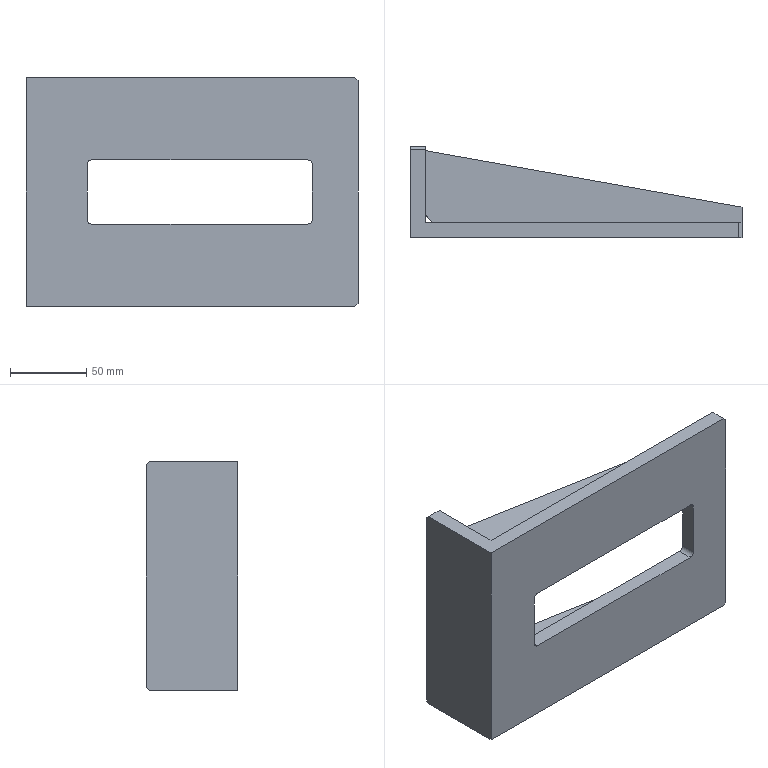Part | SolidWorks | features ICE 2, Chamfer 1, Extrusion 1, Fillet 1, MirrorPattern 1 | 1 solid | 28 faces | box 217.5 x 60 x 150 mm | volume 433717 mm3 | plane 24 | cylinder 4 | commonest cylinder face diameters 6 x4
STEP:
#1=CARTESIAN_POINT('',(0.,58.,75.));
#2=VERTEX_POINT('',#1);
#3=CARTESIAN_POINT('',(0.,0.,75.));
#4=VERTEX_POINT('',#3);
#5=CARTESIAN_POINT('',(0.,60.,75.));
#6=DIRECTION('',(0.,-1.,0.));
#7=VECTOR('',#6,1000.);
#8=LINE('',#5,#7);
#9=EDGE_CURVE('',#2,#4,#8,.T.);
#10=ORIENTED_EDGE('',*,*,#9,.F.);
#11=CARTESIAN_POINT('',(0.,60.,73.));
#12=VERTEX_POINT('',#11);
#13=CARTESIAN_POINT('',(0.,58.,75.));
#14=DIRECTION('',(0.,0.7071,-0.7071));
#15=VECTOR('',#14,1000.);
#16=LINE('',#13,#15);
#17=EDGE_CURVE('',#2,#12,#16,.T.);
#18=ORIENTED_EDGE('',*,*,#17,.T.);
#19=CARTESIAN_POINT('',(0.,60.,-73.));
#20=VERTEX_POINT('',#19);
#21=CARTESIAN_POINT('',(0.,60.,75.));
#22=DIRECTION('',(0.,0.,-1.));
#23=VECTOR('',#22,1000.);
#24=LINE('',#21,#23);
#25=EDGE_CURVE('',#12,#20,#24,.T.);
#26=ORIENTED_EDGE('',*,*,#25,.T.);
#27=CARTESIAN_POINT('',(0.,58.,-75.));
#28=VERTEX_POINT('',#27);
#29=CARTESIAN_POINT('',(0.,60.,-73.));
#30=DIRECTION('',(0.,-0.7071,-0.7071));
#31=VECTOR('',#30,1000.);
#32=LINE('',#29,#31);
#33=EDGE_CURVE('',#20,#28,#32,.T.);
#34=ORIENTED_EDGE('',*,*,#33,.T.);
#35=CARTESIAN_POINT('',(0.,0.,-75.));
#36=VERTEX_POINT('',#35);
#37=CARTESIAN_POINT('',(0.,60.,-75.));
#38=DIRECTION('',(0.,-1.,0.));
#39=VECTOR('',#38,1000.);
#40=LINE('',#37,#39);
#41=EDGE_CURVE('',#28,#36,#40,.T.);
#42=ORIENTED_EDGE('',*,*,#41,.T.);
#43=CARTESIAN_POINT('',(0.,0.,75.));
#44=DIRECTION('',(0.,0.,-1.));
#45=VECTOR('',#44,1000.);
#46=LINE('',#43,#45);
#47=EDGE_CURVE('',#4,#36,#46,.T.);
#48=ORIENTED_EDGE('',*,*,#47,.F.);
#49=EDGE_LOOP('',(#10,#18,#26,#34,#42,#48));
#50=FACE_OUTER_BOUND('',#49,.T.);
#51=CARTESIAN_POINT('',(0.,60.,75.));
#52=DIRECTION('',(1.,0.,0.));
#53=DIRECTION('',(0.,1.,0.));
#54=AXIS2_PLACEMENT_3D('',#51,#52,#53);
#55=PLANE('',#54);
#56=ADVANCED_FACE('',(#50),#55,.F.);
#57=CARTESIAN_POINT('',(184.5,0.,21.));
#58=VERTEX_POINT('',#57);
#59=CARTESIAN_POINT('',(43.,0.,21.));
#60=VERTEX_POINT('',#59);
#61=CARTESIAN_POINT('',(40.,0.,21.));
#62=DIRECTION('',(-1.,0.,0.));
#63=VECTOR('',#62,1000.);
#64=LINE('',#61,#63);
#65=EDGE_CURVE('',#58,#60,#64,.T.);
#66=ORIENTED_EDGE('',*,*,#65,.F.);
#67=CARTESIAN_POINT('',(187.5,0.,18.));
#68=VERTEX_POINT('',#67);
#69=CARTESIAN_POINT('',(184.5,0.,18.));
#70=DIRECTION('',(0.,1.,0.));
#71=DIRECTION('',(0.,0.,1.));
#72=AXIS2_PLACEMENT_3D('',#69,#70,#71);
#73=CIRCLE('',#72,3.);
#74=EDGE_CURVE('',#58,#68,#73,.T.);
#75=ORIENTED_EDGE('',*,*,#74,.T.);
#76=CARTESIAN_POINT('',(187.5,0.,-18.));
#77=VERTEX_POINT('',#76);
#78=CARTESIAN_POINT('',(187.5,0.,21.));
#79=DIRECTION('',(0.,0.,1.));
#80=VECTOR('',#79,1000.);
#81=LINE('',#78,#80);
#82=EDGE_CURVE('',#77,#68,#81,.T.);
#83=ORIENTED_EDGE('',*,*,#82,.F.);
#84=CARTESIAN_POINT('',(184.5,0.,-21.));
#85=VERTEX_POINT('',#84);
#86=CARTESIAN_POINT('',(184.5,0.,-18.));
#87=DIRECTION('',(0.,1.,0.));
#88=DIRECTION('',(0.,0.,1.));
#89=AXIS2_PLACEMENT_3D('',#86,#87,#88);
#90=CIRCLE('',#89,3.);
#91=EDGE_CURVE('',#77,#85,#90,.T.);
#92=ORIENTED_EDGE('',*,*,#91,.T.);
#93=CARTESIAN_POINT('',(43.,0.,-21.));
#94=VERTEX_POINT('',#93);
#95=CARTESIAN_POINT('',(40.,0.,-21.));
#96=DIRECTION('',(1.,0.,0.));
#97=VECTOR('',#96,1000.);
#98=LINE('',#95,#97);
#99=EDGE_CURVE('',#94,#85,#98,.T.);
#100=ORIENTED_EDGE('',*,*,#99,.F.);
#101=CARTESIAN_POINT('',(40.,0.,-18.));
#102=VERTEX_POINT('',#101);
#103=CARTESIAN_POINT('',(43.,0.,-18.));
#104=DIRECTION('',(0.,1.,0.));
#105=DIRECTION('',(0.,0.,1.));
#106=AXIS2_PLACEMENT_3D('',#103,#104,#105);
#107=CIRCLE('',#106,3.);
#108=EDGE_CURVE('',#94,#102,#107,.T.);
#109=ORIENTED_EDGE('',*,*,#108,.T.);
#110=CARTESIAN_POINT('',(40.,0.,18.));
#111=VERTEX_POINT('',#110);
#112=CARTESIAN_POINT('',(40.,0.,21.));
#113=DIRECTION('',(0.,0.,-1.));
#114=VECTOR('',#113,1000.);
#115=LINE('',#112,#114);
#116=EDGE_CURVE('',#111,#102,#115,.T.);
#117=ORIENTED_EDGE('',*,*,#116,.F.);
#118=CARTESIAN_POINT('',(43.,0.,18.));
#119=DIRECTION('',(0.,1.,0.));
#120=DIRECTION('',(0.,0.,1.));
#121=AXIS2_PLACEMENT_3D('',#118,#119,#120);
#122=CIRCLE('',#121,3.);
#123=EDGE_CURVE('',#111,#60,#122,.T.);
#124=ORIENTED_EDGE('',*,*,#123,.T.);
#125=EDGE_LOOP('',(#66,#75,#83,#92,#100,#109,#117,#124));
#126=FACE_BOUND('',#125,.T.);
#127=CARTESIAN_POINT('',(215.5,0.,-75.));
#128=VERTEX_POINT('',#127);
#129=CARTESIAN_POINT('',(0.,0.,-75.));
#130=DIRECTION('',(1.,0.,0.));
#131=VECTOR('',#130,1000.);
#132=LINE('',#129,#131);
#133=EDGE_CURVE('',#36,#128,#132,.T.);
#134=ORIENTED_EDGE('',*,*,#133,.T.);
#135=CARTESIAN_POINT('',(217.5,0.,-73.));
#136=VERTEX_POINT('',#135);
#137=CARTESIAN_POINT('',(217.5,0.,-73.));
#138=DIRECTION('',(0.7071,0.,0.7071));
#139=VECTOR('',#138,1000.);
#140=LINE('',#137,#139);
#141=EDGE_CURVE('',#128,#136,#140,.T.);
#142=ORIENTED_EDGE('',*,*,#141,.T.);
#143=CARTESIAN_POINT('',(217.5,0.,73.));
#144=VERTEX_POINT('',#143);
#145=CARTESIAN_POINT('',(217.5,0.,75.));
#146=DIRECTION('',(0.,0.,-1.));
#147=VECTOR('',#146,1000.);
#148=LINE('',#145,#147);
#149=EDGE_CURVE('',#144,#136,#148,.T.);
#150=ORIENTED_EDGE('',*,*,#149,.F.);
#151=CARTESIAN_POINT('',(215.5,0.,75.));
#152=VERTEX_POINT('',#151);
#153=CARTESIAN_POINT('',(215.5,0.,75.));
#154=DIRECTION('',(-0.7071,0.,0.7071));
#155=VECTOR('',#154,1000.);
#156=LINE('',#153,#155);
#157=EDGE_CURVE('',#144,#152,#156,.T.);
#158=ORIENTED_EDGE('',*,*,#157,.T.);
#159=CARTESIAN_POINT('',(0.,0.,75.));
#160=DIRECTION('',(1.,0.,0.));
#161=VECTOR('',#160,1000.);
#162=LINE('',#159,#161);
#163=EDGE_CURVE('',#4,#152,#162,.T.);
#164=ORIENTED_EDGE('',*,*,#163,.F.);
#165=ORIENTED_EDGE('',*,*,#47,.T.);
#166=EDGE_LOOP('',(#134,#142,#150,#158,#164,#165));
#167=FACE_OUTER_BOUND('',#166,.T.);
#168=CARTESIAN_POINT('',(0.,0.,75.));
#169=DIRECTION('',(0.,1.,0.));
#170=DIRECTION('',(0.,0.,1.));
#171=AXIS2_PLACEMENT_3D('',#168,#169,#170);
#172=PLANE('',#171);
#173=ADVANCED_FACE('',(#126,#167),#172,.F.);
#174=ORIENTED_EDGE('',*,*,#149,.T.);
#175=CARTESIAN_POINT('',(217.5,10.,-73.));
#176=VERTEX_POINT('',#175);
#177=CARTESIAN_POINT('',(217.5,0.,-73.));
#178=DIRECTION('',(0.,1.,0.));
#179=VECTOR('',#178,1000.);
#180=LINE('',#177,#179);
#181=EDGE_CURVE('',#136,#176,#180,.T.);
#182=ORIENTED_EDGE('',*,*,#181,.T.);
#183=CARTESIAN_POINT('',(217.5,10.,-54.));
#184=VERTEX_POINT('',#183);
#185=CARTESIAN_POINT('',(217.5,10.,75.));
#186=DIRECTION('',(0.,0.,-1.));
#187=VECTOR('',#186,1000.);
#188=LINE('',#185,#187);
#189=EDGE_CURVE('',#184,#176,#188,.T.);
#190=ORIENTED_EDGE('',*,*,#189,.F.);
#191=CARTESIAN_POINT('',(217.5,20.,-54.));
#192=VERTEX_POINT('',#191);
#193=CARTESIAN_POINT('',(217.5,20.,-54.));
#194=DIRECTION('',(0.,1.,0.));
#195=VECTOR('',#194,1000.);
#196=LINE('',#193,#195);
#197=EDGE_CURVE('',#184,#192,#196,.T.);
#198=ORIENTED_EDGE('',*,*,#197,.T.);
#199=CARTESIAN_POINT('',(217.5,20.,-46.));
#200=VERTEX_POINT('',#199);
#201=CARTESIAN_POINT('',(217.5,20.,-54.));
#202=DIRECTION('',(0.,0.,1.));
#203=VECTOR('',#202,1000.);
#204=LINE('',#201,#203);
#205=EDGE_CURVE('',#192,#200,#204,.T.);
#206=ORIENTED_EDGE('',*,*,#205,.T.);
#207=CARTESIAN_POINT('',(217.5,10.,-46.));
#208=VERTEX_POINT('',#207);
#209=CARTESIAN_POINT('',(217.5,20.,-46.));
#210=DIRECTION('',(0.,1.,0.));
#211=VECTOR('',#210,1000.);
#212=LINE('',#209,#211);
#213=EDGE_CURVE('',#208,#200,#212,.T.);
#214=ORIENTED_EDGE('',*,*,#213,.F.);
#215=CARTESIAN_POINT('',(217.5,10.,46.));
#216=VERTEX_POINT('',#215);
#217=CARTESIAN_POINT('',(217.5,10.,75.));
#218=DIRECTION('',(0.,0.,-1.));
#219=VECTOR('',#218,1000.);
#220=LINE('',#217,#219);
#221=EDGE_CURVE('',#216,#208,#220,.T.);
#222=ORIENTED_EDGE('',*,*,#221,.F.);
#223=CARTESIAN_POINT('',(217.5,20.,46.));
#224=VERTEX_POINT('',#223);
#225=CARTESIAN_POINT('',(217.5,20.,46.));
#226=DIRECTION('',(0.,1.,0.));
#227=VECTOR('',#226,1000.);
#228=LINE('',#225,#227);
#229=EDGE_CURVE('',#216,#224,#228,.T.);
#230=ORIENTED_EDGE('',*,*,#229,.T.);
#231=CARTESIAN_POINT('',(217.5,20.,54.));
#232=VERTEX_POINT('',#231);
#233=CARTESIAN_POINT('',(217.5,20.,54.));
#234=DIRECTION('',(0.,0.,-1.));
#235=VECTOR('',#234,1000.);
#236=LINE('',#233,#235);
#237=EDGE_CURVE('',#232,#224,#236,.T.);
#238=ORIENTED_EDGE('',*,*,#237,.F.);
#239=CARTESIAN_POINT('',(217.5,10.,54.));
#240=VERTEX_POINT('',#239);
#241=CARTESIAN_POINT('',(217.5,20.,54.));
#242=DIRECTION('',(0.,1.,0.));
#243=VECTOR('',#242,1000.);
#244=LINE('',#241,#243);
#245=EDGE_CURVE('',#240,#232,#244,.T.);
#246=ORIENTED_EDGE('',*,*,#245,.F.);
#247=CARTESIAN_POINT('',(217.5,10.,73.));
#248=VERTEX_POINT('',#247);
#249=CARTESIAN_POINT('',(217.5,10.,75.));
#250=DIRECTION('',(0.,0.,-1.));
#251=VECTOR('',#250,1000.);
#252=LINE('',#249,#251);
#253=EDGE_CURVE('',#248,#240,#252,.T.);
#254=ORIENTED_EDGE('',*,*,#253,.F.);
#255=CARTESIAN_POINT('',(217.5,0.,73.));
#256=DIRECTION('',(0.,-1.,0.));
#257=VECTOR('',#256,1000.);
#258=LINE('',#255,#257);
#259=EDGE_CURVE('',#248,#144,#258,.T.);
#260=ORIENTED_EDGE('',*,*,#259,.T.);
#261=EDGE_LOOP('',(#174,#182,#190,#198,#206,#214,#222,#230,#238,#246,#254,#260));
#262=FACE_OUTER_BOUND('',#261,.T.);
#263=CARTESIAN_POINT('',(217.5,0.,75.));
#264=DIRECTION('',(-1.,0.,0.));
#265=DIRECTION('',(0.,0.,1.));
#266=AXIS2_PLACEMENT_3D('',#263,#264,#265);
#267=PLANE('',#266);
#268=ADVANCED_FACE('',(#262),#267,.F.);
#269=CARTESIAN_POINT('',(184.5,10.,-21.));
#270=VERTEX_POINT('',#269);
#271=CARTESIAN_POINT('',(43.,10.,-21.));
#272=VERTEX_POINT('',#271);
#273=CARTESIAN_POINT('',(40.,10.,-21.));
#274=DIRECTION('',(-1.,0.,0.));
#275=VECTOR('',#274,1000.);
#276=LINE('',#273,#275);
#277=EDGE_CURVE('',#270,#272,#276,.T.);
#278=ORIENTED_EDGE('',*,*,#277,.F.);
#279=CARTESIAN_POINT('',(187.5,10.,-18.));
#280=VERTEX_POINT('',#279);
#281=CARTESIAN_POINT('',(184.5,10.,-18.));
#282=DIRECTION('',(0.,-1.,0.));
#283=DIRECTION('',(1.,0.,0.));
#284=AXIS2_PLACEMENT_3D('',#281,#282,#283);
#285=CIRCLE('',#284,3.);
#286=EDGE_CURVE('',#270,#280,#285,.T.);
#287=ORIENTED_EDGE('',*,*,#286,.T.);
#288=CARTESIAN_POINT('',(187.5,10.,18.));
#289=VERTEX_POINT('',#288);
#290=CARTESIAN_POINT('',(187.5,10.,21.));
#291=DIRECTION('',(0.,0.,-1.));
#292=VECTOR('',#291,1000.);
#293=LINE('',#290,#292);
#294=EDGE_CURVE('',#289,#280,#293,.T.);
#295=ORIENTED_EDGE('',*,*,#294,.F.);
#296=CARTESIAN_POINT('',(184.5,10.,21.));
#297=VERTEX_POINT('',#296);
#298=CARTESIAN_POINT('',(184.5,10.,18.));
#299=DIRECTION('',(0.,-1.,0.));
#300=DIRECTION('',(1.,0.,0.));
#301=AXIS2_PLACEMENT_3D('',#298,#299,#300);
#302=CIRCLE('',#301,3.);
#303=EDGE_CURVE('',#289,#297,#302,.T.);
#304=ORIENTED_EDGE('',*,*,#303,.T.);
#305=CARTESIAN_POINT('',(43.,10.,21.));
#306=VERTEX_POINT('',#305);
#307=CARTESIAN_POINT('',(40.,10.,21.));
#308=DIRECTION('',(1.,0.,0.));
#309=VECTOR('',#308,1000.);
#310=LINE('',#307,#309);
#311=EDGE_CURVE('',#306,#297,#310,.T.);
#312=ORIENTED_EDGE('',*,*,#311,.F.);
#313=CARTESIAN_POINT('',(40.,10.,18.));
#314=VERTEX_POINT('',#313);
#315=CARTESIAN_POINT('',(43.,10.,18.));
#316=DIRECTION('',(0.,-1.,0.));
#317=DIRECTION('',(1.,0.,0.));
#318=AXIS2_PLACEMENT_3D('',#315,#316,#317);
#319=CIRCLE('',#318,3.);
#320=EDGE_CURVE('',#306,#314,#319,.T.);
#321=ORIENTED_EDGE('',*,*,#320,.T.);
#322=CARTESIAN_POINT('',(40.,10.,-18.));
#323=VERTEX_POINT('',#322);
#324=CARTESIAN_POINT('',(40.,10.,21.));
#325=DIRECTION('',(0.,0.,1.));
#326=VECTOR('',#325,1000.);
#327=LINE('',#324,#326);
#328=EDGE_CURVE('',#323,#314,#327,.T.);
#329=ORIENTED_EDGE('',*,*,#328,.F.);
#330=CARTESIAN_POINT('',(43.,10.,-18.));
#331=DIRECTION('',(0.,-1.,0.));
#332=DIRECTION('',(1.,0.,0.));
#333=AXIS2_PLACEMENT_3D('',#330,#331,#332);
#334=CIRCLE('',#333,3.);
#335=EDGE_CURVE('',#323,#272,#334,.T.);
#336=ORIENTED_EDGE('',*,*,#335,.T.);
#337=EDGE_LOOP('',(#278,#287,#295,#304,#312,#321,#329,#336));
#338=FACE_BOUND('',#337,.T.);
#339=CARTESIAN_POINT('',(15.,10.,-54.));
#340=VERTEX_POINT('',#339);
#341=CARTESIAN_POINT('',(15.,10.,-46.));
#342=VERTEX_POINT('',#341);
#343=CARTESIAN_POINT('',(15.,10.,-54.));
#344=DIRECTION('',(0.,0.,1.));
#345=VECTOR('',#344,1000.);
#346=LINE('',#343,#345);
#347=EDGE_CURVE('',#340,#342,#346,.T.);
#348=ORIENTED_EDGE('',*,*,#347,.F.);
#349=CARTESIAN_POINT('',(217.5,10.,-54.));
#350=DIRECTION('',(1.,0.,0.));
#351=VECTOR('',#350,1000.);
#352=LINE('',#349,#351);
#353=EDGE_CURVE('',#340,#184,#352,.T.);
#354=ORIENTED_EDGE('',*,*,#353,.T.);
#355=ORIENTED_EDGE('',*,*,#189,.T.);
#356=CARTESIAN_POINT('',(215.5,10.,-75.));
#357=VERTEX_POINT('',#356);
#358=CARTESIAN_POINT('',(217.5,10.,-73.));
#359=DIRECTION('',(-0.7071,0.,-0.7071));
#360=VECTOR('',#359,1000.);
#361=LINE('',#358,#360);
#362=EDGE_CURVE('',#176,#357,#361,.T.);
#363=ORIENTED_EDGE('',*,*,#362,.T.);
#364=CARTESIAN_POINT('',(10.,10.,-75.));
#365=VERTEX_POINT('',#364);
#366=CARTESIAN_POINT('',(217.5,10.,-75.));
#367=DIRECTION('',(-1.,0.,0.));
#368=VECTOR('',#367,1000.);
#369=LINE('',#366,#368);
#370=EDGE_CURVE('',#357,#365,#369,.T.);
#371=ORIENTED_EDGE('',*,*,#370,.T.);
#372=CARTESIAN_POINT('',(10.,10.,75.));
#373=VERTEX_POINT('',#372);
#374=CARTESIAN_POINT('',(10.,10.,75.));
#375=DIRECTION('',(0.,0.,-1.));
#376=VECTOR('',#375,1000.);
#377=LINE('',#374,#376);
#378=EDGE_CURVE('',#373,#365,#377,.T.);
#379=ORIENTED_EDGE('',*,*,#378,.F.);
#380=CARTESIAN_POINT('',(215.5,10.,75.));
#381=VERTEX_POINT('',#380);
#382=CARTESIAN_POINT('',(217.5,10.,75.));
#383=DIRECTION('',(-1.,0.,0.));
#384=VECTOR('',#383,1000.);
#385=LINE('',#382,#384);
#386=EDGE_CURVE('',#381,#373,#385,.T.);
#387=ORIENTED_EDGE('',*,*,#386,.F.);
#388=CARTESIAN_POINT('',(215.5,10.,75.));
#389=DIRECTION('',(0.7071,0.,-0.7071));
#390=VECTOR('',#389,1000.);
#391=LINE('',#388,#390);
#392=EDGE_CURVE('',#381,#248,#391,.T.);
#393=ORIENTED_EDGE('',*,*,#392,.T.);
#394=ORIENTED_EDGE('',*,*,#253,.T.);
#395=CARTESIAN_POINT('',(15.,10.,54.));
#396=VERTEX_POINT('',#395);
#397=CARTESIAN_POINT('',(217.5,10.,54.));
#398=DIRECTION('',(1.,0.,0.));
#399=VECTOR('',#398,1000.);
#400=LINE('',#397,#399);
#401=EDGE_CURVE('',#396,#240,#400,.T.);
#402=ORIENTED_EDGE('',*,*,#401,.F.);
#403=CARTESIAN_POINT('',(15.,10.,46.));
#404=VERTEX_POINT('',#403);
#405=CARTESIAN_POINT('',(15.,10.,54.));
#406=DIRECTION('',(0.,0.,-1.));
#407=VECTOR('',#406,1000.);
#408=LINE('',#405,#407);
#409=EDGE_CURVE('',#396,#404,#408,.T.);
#410=ORIENTED_EDGE('',*,*,#409,.T.);
#411=CARTESIAN_POINT('',(217.5,10.,46.));
#412=DIRECTION('',(1.,0.,0.));
#413=VECTOR('',#412,1000.);
#414=LINE('',#411,#413);
#415=EDGE_CURVE('',#404,#216,#414,.T.);
#416=ORIENTED_EDGE('',*,*,#415,.T.);
#417=ORIENTED_EDGE('',*,*,#221,.T.);
#418=CARTESIAN_POINT('',(217.5,10.,-46.));
#419=DIRECTION('',(1.,0.,0.));
#420=VECTOR('',#419,1000.);
#421=LINE('',#418,#420);
#422=EDGE_CURVE('',#342,#208,#421,.T.);
#423=ORIENTED_EDGE('',*,*,#422,.F.);
#424=EDGE_LOOP('',(#348,#354,#355,#363,#371,#379,#387,#393,#394,#402,#410,#416,#417,#423));
#425=FACE_OUTER_BOUND('',#424,.T.);
#426=CARTESIAN_POINT('',(217.5,10.,75.));
#427=DIRECTION('',(0.,-1.,0.));
#428=DIRECTION('',(1.,0.,0.));
#429=AXIS2_PLACEMENT_3D('',#426,#427,#428);
#430=PLANE('',#429);
#431=ADVANCED_FACE('',(#338,#425),#430,.F.);
#432=CARTESIAN_POINT('',(10.,57.,-54.));
#433=VERTEX_POINT('',#432);
#434=CARTESIAN_POINT('',(10.,57.,-46.));
#435=VERTEX_POINT('',#434);
#436=CARTESIAN_POINT('',(10.,57.,-54.));
#437=DIRECTION('',(0.,0.,1.));
#438=VECTOR('',#437,1000.);
#439=LINE('',#436,#438);
#440=EDGE_CURVE('',#433,#435,#439,.T.);
#441=ORIENTED_EDGE('',*,*,#440,.F.);
#442=CARTESIAN_POINT('',(10.,15.,-54.));
#443=VERTEX_POINT('',#442);
#444=CARTESIAN_POINT('',(10.,15.,-54.));
#445=DIRECTION('',(0.,-1.,0.));
#446=VECTOR('',#445,1000.);
#447=LINE('',#444,#446);
#448=EDGE_CURVE('',#433,#443,#447,.T.);
#449=ORIENTED_EDGE('',*,*,#448,.T.);
#450=CARTESIAN_POINT('',(10.,15.,-46.));
#451=VERTEX_POINT('',#450);
#452=CARTESIAN_POINT('',(10.,15.,-54.));
#453=DIRECTION('',(0.,0.,1.));
#454=VECTOR('',#453,1000.);
#455=LINE('',#452,#454);
#456=EDGE_CURVE('',#443,#451,#455,.T.);
#457=ORIENTED_EDGE('',*,*,#456,.T.);
#458=CARTESIAN_POINT('',(10.,15.,-46.));
#459=DIRECTION('',(0.,-1.,0.));
#460=VECTOR('',#459,1000.);
#461=LINE('',#458,#460);
#462=EDGE_CURVE('',#435,#451,#461,.T.);
#463=ORIENTED_EDGE('',*,*,#462,.F.);
#464=EDGE_LOOP('',(#441,#449,#457,#463));
#465=FACE_BOUND('',#464,.T.);
#466=CARTESIAN_POINT('',(10.,15.,54.));
#467=VERTEX_POINT('',#466);
#468=CARTESIAN_POINT('',(10.,15.,46.));
#469=VERTEX_POINT('',#468);
#470=CARTESIAN_POINT('',(10.,15.,54.));
#471=DIRECTION('',(0.,0.,-1.));
#472=VECTOR('',#471,1000.);
#473=LINE('',#470,#472);
#474=EDGE_CURVE('',#467,#469,#473,.T.);
#475=ORIENTED_EDGE('',*,*,#474,.F.);
#476=CARTESIAN_POINT('',(10.,57.,54.));
#477=VERTEX_POINT('',#476);
#478=CARTESIAN_POINT('',(10.,15.,54.));
#479=DIRECTION('',(0.,-1.,0.));
#480=VECTOR('',#479,1000.);
#481=LINE('',#478,#480);
#482=EDGE_CURVE('',#477,#467,#481,.T.);
#483=ORIENTED_EDGE('',*,*,#482,.F.);
#484=CARTESIAN_POINT('',(10.,57.,46.));
#485=VERTEX_POINT('',#484);
#486=CARTESIAN_POINT('',(10.,57.,54.));
#487=DIRECTION('',(0.,0.,-1.));
#488=VECTOR('',#487,1000.);
#489=LINE('',#486,#488);
#490=EDGE_CURVE('',#477,#485,#489,.T.);
#491=ORIENTED_EDGE('',*,*,#490,.T.);
#492=CARTESIAN_POINT('',(10.,15.,46.));
#493=DIRECTION('',(0.,-1.,0.));
#494=VECTOR('',#493,1000.);
#495=LINE('',#492,#494);
#496=EDGE_CURVE('',#485,#469,#495,.T.);
#497=ORIENTED_EDGE('',*,*,#496,.T.);
#498=EDGE_LOOP('',(#475,#483,#491,#497));
#499=FACE_BOUND('',#498,.T.);
#500=CARTESIAN_POINT('',(10.,60.,73.));
#501=VERTEX_POINT('',#500);
#502=CARTESIAN_POINT('',(10.,60.,-73.));
#503=VERTEX_POINT('',#502);
#504=CARTESIAN_POINT('',(10.,60.,75.));
#505=DIRECTION('',(0.,0.,-1.));
#506=VECTOR('',#505,1000.);
#507=LINE('',#504,#506);
#508=EDGE_CURVE('',#501,#503,#507,.T.);
#509=ORIENTED_EDGE('',*,*,#508,.F.);
#510=CARTESIAN_POINT('',(10.,58.,75.));
#511=VERTEX_POINT('',#510);
#512=CARTESIAN_POINT('',(10.,58.,75.));
#513=DIRECTION('',(0.,-0.7071,0.7071));
#514=VECTOR('',#513,1000.);
#515=LINE('',#512,#514);
#516=EDGE_CURVE('',#501,#511,#515,.T.);
#517=ORIENTED_EDGE('',*,*,#516,.T.);
#518=CARTESIAN_POINT('',(10.,10.,75.));
#519=DIRECTION('',(0.,1.,0.));
#520=VECTOR('',#519,1000.);
#521=LINE('',#518,#520);
#522=EDGE_CURVE('',#373,#511,#521,.T.);
#523=ORIENTED_EDGE('',*,*,#522,.F.);
#524=ORIENTED_EDGE('',*,*,#378,.T.);
#525=CARTESIAN_POINT('',(10.,58.,-75.));
#526=VERTEX_POINT('',#525);
#527=CARTESIAN_POINT('',(10.,10.,-75.));
#528=DIRECTION('',(0.,1.,0.));
#529=VECTOR('',#528,1000.);
#530=LINE('',#527,#529);
#531=EDGE_CURVE('',#365,#526,#530,.T.);
#532=ORIENTED_EDGE('',*,*,#531,.T.);
#533=CARTESIAN_POINT('',(10.,60.,-73.));
#534=DIRECTION('',(0.,0.7071,0.7071));
#535=VECTOR('',#534,1000.);
#536=LINE('',#533,#535);
#537=EDGE_CURVE('',#526,#503,#536,.T.);
#538=ORIENTED_EDGE('',*,*,#537,.T.);
#539=EDGE_LOOP('',(#509,#517,#523,#524,#532,#538));
#540=FACE_OUTER_BOUND('',#539,.T.);
#541=CARTESIAN_POINT('',(10.,10.,75.));
#542=DIRECTION('',(-1.,0.,0.));
#543=DIRECTION('',(0.,-1.,0.));
#544=AXIS2_PLACEMENT_3D('',#541,#542,#543);
#545=PLANE('',#544);
#546=ADVANCED_FACE('',(#465,#499,#540),#545,.F.);
#547=ORIENTED_EDGE('',*,*,#25,.F.);
#548=CARTESIAN_POINT('',(10.,60.,73.));
#549=DIRECTION('',(1.,0.,0.));
#550=VECTOR('',#549,1000.);
#551=LINE('',#548,#550);
#552=EDGE_CURVE('',#12,#501,#551,.T.);
#553=ORIENTED_EDGE('',*,*,#552,.T.);
#554=ORIENTED_EDGE('',*,*,#508,.T.);
#555=CARTESIAN_POINT('',(10.,60.,-73.));
#556=DIRECTION('',(-1.,0.,0.));
#557=VECTOR('',#556,1000.);
#558=LINE('',#555,#557);
#559=EDGE_CURVE('',#503,#20,#558,.T.);
#560=ORIENTED_EDGE('',*,*,#559,.T.);
#561=EDGE_LOOP('',(#547,#553,#554,#560));
#562=FACE_OUTER_BOUND('',#561,.T.);
#563=CARTESIAN_POINT('',(10.,60.,75.));
#564=DIRECTION('',(0.,-1.,0.));
#565=DIRECTION('',(0.,0.,-1.));
#566=AXIS2_PLACEMENT_3D('',#563,#564,#565);
#567=PLANE('',#566);
#568=ADVANCED_FACE('',(#562),#567,.F.);
#569=ORIENTED_EDGE('',*,*,#163,.T.);
#570=CARTESIAN_POINT('',(215.5,10.,75.));
#571=DIRECTION('',(0.,1.,0.));
#572=VECTOR('',#571,1000.);
#573=LINE('',#570,#572);
#574=EDGE_CURVE('',#152,#381,#573,.T.);
#575=ORIENTED_EDGE('',*,*,#574,.T.);
#576=ORIENTED_EDGE('',*,*,#386,.T.);
#577=ORIENTED_EDGE('',*,*,#522,.T.);
#578=CARTESIAN_POINT('',(0.,58.,75.));
#579=DIRECTION('',(-1.,0.,0.));
#580=VECTOR('',#579,1000.);
#581=LINE('',#578,#580);
#582=EDGE_CURVE('',#511,#2,#581,.T.);
#583=ORIENTED_EDGE('',*,*,#582,.T.);
#584=ORIENTED_EDGE('',*,*,#9,.T.);
#585=EDGE_LOOP('',(#569,#575,#576,#577,#583,#584));
#586=FACE_OUTER_BOUND('',#585,.T.);
#587=CARTESIAN_POINT('',(0.,0.,75.));
#588=DIRECTION('',(0.,0.,1.));
#589=DIRECTION('',(1.,0.,0.));
#590=AXIS2_PLACEMENT_3D('',#587,#588,#589);
#591=PLANE('',#590);
#592=ADVANCED_FACE('',(#586),#591,.T.);
#593=ORIENTED_EDGE('',*,*,#370,.F.);
#594=CARTESIAN_POINT('',(215.5,0.,-75.));
#595=DIRECTION('',(0.,-1.,0.));
#596=VECTOR('',#595,1000.);
#597=LINE('',#594,#596);
#598=EDGE_CURVE('',#357,#128,#597,.T.);
#599=ORIENTED_EDGE('',*,*,#598,.T.);
#600=ORIENTED_EDGE('',*,*,#133,.F.);
#601=ORIENTED_EDGE('',*,*,#41,.F.);
#602=CARTESIAN_POINT('',(0.,58.,-75.));
#603=DIRECTION('',(1.,0.,0.));
#604=VECTOR('',#603,1000.);
#605=LINE('',#602,#604);
#606=EDGE_CURVE('',#28,#526,#605,.T.);
#607=ORIENTED_EDGE('',*,*,#606,.T.);
#608=ORIENTED_EDGE('',*,*,#531,.F.);
#609=EDGE_LOOP('',(#593,#599,#600,#601,#607,#608));
#610=FACE_OUTER_BOUND('',#609,.T.);
#611=CARTESIAN_POINT('',(0.,0.,-75.));
#612=DIRECTION('',(0.,0.,1.));
#613=DIRECTION('',(1.,0.,0.));
#614=AXIS2_PLACEMENT_3D('',#611,#612,#613);
#615=PLANE('',#614);
#616=ADVANCED_FACE('',(#610),#615,.F.);
#617=CARTESIAN_POINT('',(15.,10.,46.));
#618=DIRECTION('',(0.7071,-0.7071,0.));
#619=VECTOR('',#618,1000.);
#620=LINE('',#617,#619);
#621=EDGE_CURVE('',#469,#404,#620,.T.);
#622=ORIENTED_EDGE('',*,*,#621,.T.);
#623=ORIENTED_EDGE('',*,*,#409,.F.);
#624=CARTESIAN_POINT('',(15.,10.,54.));
#625=DIRECTION('',(0.7071,-0.7071,0.));
#626=VECTOR('',#625,1000.);
#627=LINE('',#624,#626);
#628=EDGE_CURVE('',#467,#396,#627,.T.);
#629=ORIENTED_EDGE('',*,*,#628,.F.);
#630=ORIENTED_EDGE('',*,*,#474,.T.);
#631=EDGE_LOOP('',(#622,#623,#629,#630));
#632=FACE_OUTER_BOUND('',#631,.T.);
#633=CARTESIAN_POINT('',(15.,10.,54.));
#634=DIRECTION('',(0.7071,0.7071,0.));
#635=DIRECTION('',(-0.7071,0.7071,0.));
#636=AXIS2_PLACEMENT_3D('',#633,#634,#635);
#637=PLANE('',#636);
#638=ADVANCED_FACE('',(#632),#637,.F.);
#639=CARTESIAN_POINT('',(10.,57.,46.));
#640=DIRECTION('',(-0.9845,0.1755,0.));
#641=VECTOR('',#640,1000.);
#642=LINE('',#639,#641);
#643=EDGE_CURVE('',#224,#485,#642,.T.);
#644=ORIENTED_EDGE('',*,*,#643,.T.);
#645=ORIENTED_EDGE('',*,*,#490,.F.);
#646=CARTESIAN_POINT('',(10.,57.,54.));
#647=DIRECTION('',(-0.9845,0.1755,0.));
#648=VECTOR('',#647,1000.);
#649=LINE('',#646,#648);
#650=EDGE_CURVE('',#232,#477,#649,.T.);
#651=ORIENTED_EDGE('',*,*,#650,.F.);
#652=ORIENTED_EDGE('',*,*,#237,.T.);
#653=EDGE_LOOP('',(#644,#645,#651,#652));
#654=FACE_OUTER_BOUND('',#653,.T.);
#655=CARTESIAN_POINT('',(10.,57.,54.));
#656=DIRECTION('',(-0.1755,-0.9845,0.));
#657=DIRECTION('',(0.9845,-0.1755,0.));
#658=AXIS2_PLACEMENT_3D('',#655,#656,#657);
#659=PLANE('',#658);
#660=ADVANCED_FACE('',(#654),#659,.F.);
#661=ORIENTED_EDGE('',*,*,#482,.T.);
#662=ORIENTED_EDGE('',*,*,#628,.T.);
#663=ORIENTED_EDGE('',*,*,#401,.T.);
#664=ORIENTED_EDGE('',*,*,#245,.T.);
#665=ORIENTED_EDGE('',*,*,#650,.T.);
#666=EDGE_LOOP('',(#661,#662,#663,#664,#665));
#667=FACE_OUTER_BOUND('',#666,.T.);
#668=CARTESIAN_POINT('',(0.,0.,54.));
#669=DIRECTION('',(0.,0.,1.));
#670=DIRECTION('',(1.,0.,0.));
#671=AXIS2_PLACEMENT_3D('',#668,#669,#670);
#672=PLANE('',#671);
#673=ADVANCED_FACE('',(#667),#672,.T.);
#674=ORIENTED_EDGE('',*,*,#496,.F.);
#675=ORIENTED_EDGE('',*,*,#643,.F.);
#676=ORIENTED_EDGE('',*,*,#229,.F.);
#677=ORIENTED_EDGE('',*,*,#415,.F.);
#678=ORIENTED_EDGE('',*,*,#621,.F.);
#679=EDGE_LOOP('',(#674,#675,#676,#677,#678));
#680=FACE_OUTER_BOUND('',#679,.T.);
#681=CARTESIAN_POINT('',(0.,0.,46.));
#682=DIRECTION('',(0.,0.,1.));
#683=DIRECTION('',(1.,0.,0.));
#684=AXIS2_PLACEMENT_3D('',#681,#682,#683);
#685=PLANE('',#684);
#686=ADVANCED_FACE('',(#680),#685,.F.);
#687=ORIENTED_EDGE('',*,*,#141,.F.);
#688=ORIENTED_EDGE('',*,*,#598,.F.);
#689=ORIENTED_EDGE('',*,*,#362,.F.);
#690=ORIENTED_EDGE('',*,*,#181,.F.);
#691=EDGE_LOOP('',(#687,#688,#689,#690));
#692=FACE_OUTER_BOUND('',#691,.T.);
#693=CARTESIAN_POINT('',(217.5,0.,-73.));
#694=DIRECTION('',(-0.7071,0.,0.7071));
#695=DIRECTION('',(0.,1.,0.));
#696=AXIS2_PLACEMENT_3D('',#693,#694,#695);
#697=PLANE('',#696);
#698=ADVANCED_FACE('',(#692),#697,.F.);
#699=ORIENTED_EDGE('',*,*,#157,.F.);
#700=ORIENTED_EDGE('',*,*,#259,.F.);
#701=ORIENTED_EDGE('',*,*,#392,.F.);
#702=ORIENTED_EDGE('',*,*,#574,.F.);
#703=EDGE_LOOP('',(#699,#700,#701,#702));
#704=FACE_OUTER_BOUND('',#703,.T.);
#705=CARTESIAN_POINT('',(215.5,0.,75.));
#706=DIRECTION('',(0.7071,0.,0.7071));
#707=DIRECTION('',(0.,-1.,0.));
#708=AXIS2_PLACEMENT_3D('',#705,#706,#707);
#709=PLANE('',#708);
#710=ADVANCED_FACE('',(#704),#709,.T.);
#711=ORIENTED_EDGE('',*,*,#516,.F.);
#712=ORIENTED_EDGE('',*,*,#552,.F.);
#713=ORIENTED_EDGE('',*,*,#17,.F.);
#714=ORIENTED_EDGE('',*,*,#582,.F.);
#715=EDGE_LOOP('',(#711,#712,#713,#714));
#716=FACE_OUTER_BOUND('',#715,.T.);
#717=CARTESIAN_POINT('',(0.,58.,75.));
#718=DIRECTION('',(0.,0.7071,0.7071));
#719=DIRECTION('',(1.,0.,0.));
#720=AXIS2_PLACEMENT_3D('',#717,#718,#719);
#721=PLANE('',#720);
#722=ADVANCED_FACE('',(#716),#721,.T.);
#723=ORIENTED_EDGE('',*,*,#537,.F.);
#724=ORIENTED_EDGE('',*,*,#606,.F.);
#725=ORIENTED_EDGE('',*,*,#33,.F.);
#726=ORIENTED_EDGE('',*,*,#559,.F.);
#727=EDGE_LOOP('',(#723,#724,#725,#726));
#728=FACE_OUTER_BOUND('',#727,.T.);
#729=CARTESIAN_POINT('',(10.,60.,-73.));
#730=DIRECTION('',(0.,-0.7071,0.7071));
#731=DIRECTION('',(-1.,0.,0.));
#732=AXIS2_PLACEMENT_3D('',#729,#730,#731);
#733=PLANE('',#732);
#734=ADVANCED_FACE('',(#728),#733,.F.);
#735=CARTESIAN_POINT('',(10.,57.,-46.));
#736=DIRECTION('',(-0.9845,0.1755,0.));
#737=VECTOR('',#736,1000.);
#738=LINE('',#735,#737);
#739=EDGE_CURVE('',#200,#435,#738,.T.);
#740=ORIENTED_EDGE('',*,*,#739,.F.);
#741=ORIENTED_EDGE('',*,*,#205,.F.);
#742=CARTESIAN_POINT('',(10.,57.,-54.));
#743=DIRECTION('',(-0.9845,0.1755,0.));
#744=VECTOR('',#743,1000.);
#745=LINE('',#742,#744);
#746=EDGE_CURVE('',#192,#433,#745,.T.);
#747=ORIENTED_EDGE('',*,*,#746,.T.);
#748=ORIENTED_EDGE('',*,*,#440,.T.);
#749=EDGE_LOOP('',(#740,#741,#747,#748));
#750=FACE_OUTER_BOUND('',#749,.T.);
#751=CARTESIAN_POINT('',(10.,57.,-54.));
#752=DIRECTION('',(0.1755,0.9845,0.));
#753=DIRECTION('',(-0.9845,0.1755,0.));
#754=AXIS2_PLACEMENT_3D('',#751,#752,#753);
#755=PLANE('',#754);
#756=ADVANCED_FACE('',(#750),#755,.T.);
#757=CARTESIAN_POINT('',(15.,10.,-46.));
#758=DIRECTION('',(0.7071,-0.7071,0.));
#759=VECTOR('',#758,1000.);
#760=LINE('',#757,#759);
#761=EDGE_CURVE('',#451,#342,#760,.T.);
#762=ORIENTED_EDGE('',*,*,#761,.F.);
#763=ORIENTED_EDGE('',*,*,#456,.F.);
#764=CARTESIAN_POINT('',(15.,10.,-54.));
#765=DIRECTION('',(0.7071,-0.7071,0.));
#766=VECTOR('',#765,1000.);
#767=LINE('',#764,#766);
#768=EDGE_CURVE('',#443,#340,#767,.T.);
#769=ORIENTED_EDGE('',*,*,#768,.T.);
#770=ORIENTED_EDGE('',*,*,#347,.T.);
#771=EDGE_LOOP('',(#762,#763,#769,#770));
#772=FACE_OUTER_BOUND('',#771,.T.);
#773=CARTESIAN_POINT('',(15.,10.,-54.));
#774=DIRECTION('',(-0.7071,-0.7071,0.));
#775=DIRECTION('',(0.7071,-0.7071,0.));
#776=AXIS2_PLACEMENT_3D('',#773,#774,#775);
#777=PLANE('',#776);
#778=ADVANCED_FACE('',(#772),#777,.T.);
#779=ORIENTED_EDGE('',*,*,#448,.F.);
#780=ORIENTED_EDGE('',*,*,#746,.F.);
#781=ORIENTED_EDGE('',*,*,#197,.F.);
#782=ORIENTED_EDGE('',*,*,#353,.F.);
#783=ORIENTED_EDGE('',*,*,#768,.F.);
#784=EDGE_LOOP('',(#779,#780,#781,#782,#783));
#785=FACE_OUTER_BOUND('',#784,.T.);
#786=CARTESIAN_POINT('',(0.,0.,-54.));
#787=DIRECTION('',(0.,0.,-1.));
#788=DIRECTION('',(1.,0.,0.));
#789=AXIS2_PLACEMENT_3D('',#786,#787,#788);
#790=PLANE('',#789);
#791=ADVANCED_FACE('',(#785),#790,.T.);
#792=ORIENTED_EDGE('',*,*,#462,.T.);
#793=ORIENTED_EDGE('',*,*,#761,.T.);
#794=ORIENTED_EDGE('',*,*,#422,.T.);
#795=ORIENTED_EDGE('',*,*,#213,.T.);
#796=ORIENTED_EDGE('',*,*,#739,.T.);
#797=EDGE_LOOP('',(#792,#793,#794,#795,#796));
#798=FACE_OUTER_BOUND('',#797,.T.);
#799=CARTESIAN_POINT('',(0.,0.,-46.));
#800=DIRECTION('',(0.,0.,-1.));
#801=DIRECTION('',(1.,0.,0.));
#802=AXIS2_PLACEMENT_3D('',#799,#800,#801);
#803=PLANE('',#802);
#804=ADVANCED_FACE('',(#798),#803,.F.);
#805=ORIENTED_EDGE('',*,*,#294,.T.);
#806=CARTESIAN_POINT('',(187.5,0.,-18.));
#807=DIRECTION('',(0.,-1.,0.));
#808=VECTOR('',#807,1000.);
#809=LINE('',#806,#808);
#810=EDGE_CURVE('',#280,#77,#809,.T.);
#811=ORIENTED_EDGE('',*,*,#810,.T.);
#812=ORIENTED_EDGE('',*,*,#82,.T.);
#813=CARTESIAN_POINT('',(187.5,10.,18.));
#814=DIRECTION('',(0.,1.,0.));
#815=VECTOR('',#814,1000.);
#816=LINE('',#813,#815);
#817=EDGE_CURVE('',#68,#289,#816,.T.);
#818=ORIENTED_EDGE('',*,*,#817,.T.);
#819=EDGE_LOOP('',(#805,#811,#812,#818));
#820=FACE_OUTER_BOUND('',#819,.T.);
#821=CARTESIAN_POINT('',(187.5,-0.001,21.));
#822=DIRECTION('',(1.,0.,0.));
#823=DIRECTION('',(0.,1.,0.));
#824=AXIS2_PLACEMENT_3D('',#821,#822,#823);
#825=PLANE('',#824);
#826=ADVANCED_FACE('',(#820),#825,.F.);
#827=ORIENTED_EDGE('',*,*,#65,.T.);
#828=CARTESIAN_POINT('',(43.,10.,21.));
#829=DIRECTION('',(0.,1.,0.));
#830=VECTOR('',#829,1000.);
#831=LINE('',#828,#830);
#832=EDGE_CURVE('',#60,#306,#831,.T.);
#833=ORIENTED_EDGE('',*,*,#832,.T.);
#834=ORIENTED_EDGE('',*,*,#311,.T.);
#835=CARTESIAN_POINT('',(184.5,0.,21.));
#836=DIRECTION('',(0.,-1.,0.));
#837=VECTOR('',#836,1000.);
#838=LINE('',#835,#837);
#839=EDGE_CURVE('',#297,#58,#838,.T.);
#840=ORIENTED_EDGE('',*,*,#839,.T.);
#841=EDGE_LOOP('',(#827,#833,#834,#840));
#842=FACE_OUTER_BOUND('',#841,.T.);
#843=CARTESIAN_POINT('',(40.,-0.001,21.));
#844=DIRECTION('',(0.,0.,1.));
#845=DIRECTION('',(1.,0.,0.));
#846=AXIS2_PLACEMENT_3D('',#843,#844,#845);
#847=PLANE('',#846);
#848=ADVANCED_FACE('',(#842),#847,.F.);
#849=ORIENTED_EDGE('',*,*,#328,.T.);
#850=CARTESIAN_POINT('',(40.,0.,18.));
#851=DIRECTION('',(0.,-1.,0.));
#852=VECTOR('',#851,1000.);
#853=LINE('',#850,#852);
#854=EDGE_CURVE('',#314,#111,#853,.T.);
#855=ORIENTED_EDGE('',*,*,#854,.T.);
#856=ORIENTED_EDGE('',*,*,#116,.T.);
#857=CARTESIAN_POINT('',(40.,10.,-18.));
#858=DIRECTION('',(0.,1.,0.));
#859=VECTOR('',#858,1000.);
#860=LINE('',#857,#859);
#861=EDGE_CURVE('',#102,#323,#860,.T.);
#862=ORIENTED_EDGE('',*,*,#861,.T.);
#863=EDGE_LOOP('',(#849,#855,#856,#862));
#864=FACE_OUTER_BOUND('',#863,.T.);
#865=CARTESIAN_POINT('',(40.,-0.001,21.));
#866=DIRECTION('',(-1.,0.,0.));
#867=DIRECTION('',(0.,-1.,0.));
#868=AXIS2_PLACEMENT_3D('',#865,#866,#867);
#869=PLANE('',#868);
#870=ADVANCED_FACE('',(#864),#869,.F.);
#871=ORIENTED_EDGE('',*,*,#99,.T.);
#872=CARTESIAN_POINT('',(184.5,10.,-21.));
#873=DIRECTION('',(0.,1.,0.));
#874=VECTOR('',#873,1000.);
#875=LINE('',#872,#874);
#876=EDGE_CURVE('',#85,#270,#875,.T.);
#877=ORIENTED_EDGE('',*,*,#876,.T.);
#878=ORIENTED_EDGE('',*,*,#277,.T.);
#879=CARTESIAN_POINT('',(43.,0.,-21.));
#880=DIRECTION('',(0.,-1.,0.));
#881=VECTOR('',#880,1000.);
#882=LINE('',#879,#881);
#883=EDGE_CURVE('',#272,#94,#882,.T.);
#884=ORIENTED_EDGE('',*,*,#883,.T.);
#885=EDGE_LOOP('',(#871,#877,#878,#884));
#886=FACE_OUTER_BOUND('',#885,.T.);
#887=CARTESIAN_POINT('',(40.,-0.001,-21.));
#888=DIRECTION('',(0.,0.,-1.));
#889=DIRECTION('',(-1.,0.,0.));
#890=AXIS2_PLACEMENT_3D('',#887,#888,#889);
#891=PLANE('',#890);
#892=ADVANCED_FACE('',(#886),#891,.F.);
#893=ORIENTED_EDGE('',*,*,#123,.F.);
#894=ORIENTED_EDGE('',*,*,#854,.F.);
#895=ORIENTED_EDGE('',*,*,#320,.F.);
#896=ORIENTED_EDGE('',*,*,#832,.F.);
#897=EDGE_LOOP('',(#893,#894,#895,#896));
#898=FACE_OUTER_BOUND('',#897,.T.);
#899=CARTESIAN_POINT('',(43.,-0.001,18.));
#900=DIRECTION('',(0.,-1.,0.));
#901=DIRECTION('',(1.,0.,0.));
#902=AXIS2_PLACEMENT_3D('',#899,#900,#901);
#903=CYLINDRICAL_SURFACE('',#902,3.);
#904=ADVANCED_FACE('',(#898),#903,.F.);
#905=ORIENTED_EDGE('',*,*,#91,.F.);
#906=ORIENTED_EDGE('',*,*,#810,.F.);
#907=ORIENTED_EDGE('',*,*,#286,.F.);
#908=ORIENTED_EDGE('',*,*,#876,.F.);
#909=EDGE_LOOP('',(#905,#906,#907,#908));
#910=FACE_OUTER_BOUND('',#909,.T.);
#911=CARTESIAN_POINT('',(184.5,-0.001,-18.));
#912=DIRECTION('',(0.,-1.,0.));
#913=DIRECTION('',(1.,0.,0.));
#914=AXIS2_PLACEMENT_3D('',#911,#912,#913);
#915=CYLINDRICAL_SURFACE('',#914,3.);
#916=ADVANCED_FACE('',(#910),#915,.F.);
#917=ORIENTED_EDGE('',*,*,#74,.F.);
#918=ORIENTED_EDGE('',*,*,#839,.F.);
#919=ORIENTED_EDGE('',*,*,#303,.F.);
#920=ORIENTED_EDGE('',*,*,#817,.F.);
#921=EDGE_LOOP('',(#917,#918,#919,#920));
#922=FACE_OUTER_BOUND('',#921,.T.);
#923=CARTESIAN_POINT('',(184.5,-0.001,18.));
#924=DIRECTION('',(0.,-1.,0.));
#925=DIRECTION('',(1.,0.,0.));
#926=AXIS2_PLACEMENT_3D('',#923,#924,#925);
#927=CYLINDRICAL_SURFACE('',#926,3.);
#928=ADVANCED_FACE('',(#922),#927,.F.);
#929=ORIENTED_EDGE('',*,*,#108,.F.);
#930=ORIENTED_EDGE('',*,*,#883,.F.);
#931=ORIENTED_EDGE('',*,*,#335,.F.);
#932=ORIENTED_EDGE('',*,*,#861,.F.);
#933=EDGE_LOOP('',(#929,#930,#931,#932));
#934=FACE_OUTER_BOUND('',#933,.T.);
#935=CARTESIAN_POINT('',(43.,-0.001,-18.));
#936=DIRECTION('',(0.,-1.,0.));
#937=DIRECTION('',(1.,0.,0.));
#938=AXIS2_PLACEMENT_3D('',#935,#936,#937);
#939=CYLINDRICAL_SURFACE('',#938,3.);
#940=ADVANCED_FACE('',(#934),#939,.F.);
#941=CLOSED_SHELL('',(#56,#173,#268,#431,#546,#568,#592,#616,#638,#660,#673,#686,#698,#710,#722,#734,#756,#778,#791,#804,#826,#848,#870,#892,#904,#916,#928,#940));
#942=MANIFOLD_SOLID_BREP('',#941);
#943=CARTESIAN_POINT('',(0.,0.,0.));
#944=DIRECTION('',(0.,0.,1.));
#945=DIRECTION('',(1.,0.,0.));
#946=AXIS2_PLACEMENT_3D('',#943,#944,#945);
#947=(LENGTH_UNIT()NAMED_UNIT(*)SI_UNIT(.MILLI.,.METRE.));
#948=UNCERTAINTY_MEASURE_WITH_UNIT(LENGTH_MEASURE(0.00001),#947,'','');
#949=(NAMED_UNIT(*)PLANE_ANGLE_UNIT()SI_UNIT($,.RADIAN.));
#950=(NAMED_UNIT(*)SI_UNIT($,.STERADIAN.)SOLID_ANGLE_UNIT());
#951=(GEOMETRIC_REPRESENTATION_CONTEXT(3)GLOBAL_UNCERTAINTY_ASSIGNED_CONTEXT((#948))GLOBAL_UNIT_ASSIGNED_CONTEXT((#947,#949,#950))REPRESENTATION_CONTEXT('',''));
#952=ADVANCED_BREP_SHAPE_REPRESENTATION('',(#942,#946),#951);